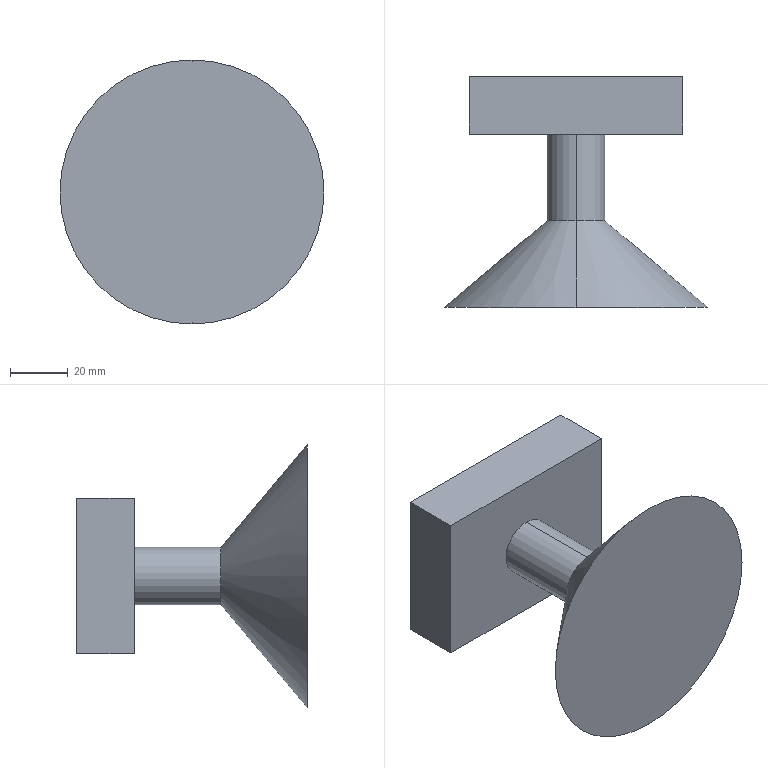Part | STEP file | Guide wheel mechanism revised.sldasm-Part-13 | 1 solid | 11 faces | box 91.505 x 80 x 91.505 mm | volume 172572 mm3 | plane 7 | cone 2 | cylinder 2 | commonest cylinder face diameters 20 x2
STEP:
#1=CARTESIAN_POINT('',(-444.995,-30.,-485.005));
#2=VERTEX_POINT('',#1);
#3=CARTESIAN_POINT('',(-444.995,-30.,-465.005));
#4=VERTEX_POINT('',#3);
#5=CARTESIAN_POINT('',(-444.995,-30.,-475.005));
#6=DIRECTION('',(0.,-1.,0.));
#7=DIRECTION('',(0.,0.,-1.));
#8=AXIS2_PLACEMENT_3D('',#5,#6,#7);
#9=CIRCLE('',#8,10.);
#10=EDGE_CURVE('',#2,#4,#9,.T.);
#11=ORIENTED_EDGE('',*,*,#10,.T.);
#12=CARTESIAN_POINT('',(-444.995,-60.,-429.252));
#13=VERTEX_POINT('',#12);
#14=CARTESIAN_POINT('',(-444.995,-30.,-465.005));
#15=DIRECTION('',(0.,-0.6428,0.766));
#16=VECTOR('',#15,1000.);
#17=LINE('',#14,#16);
#18=EDGE_CURVE('',#4,#13,#17,.T.);
#19=ORIENTED_EDGE('',*,*,#18,.T.);
#20=CARTESIAN_POINT('',(-444.995,-60.,-520.758));
#21=VERTEX_POINT('',#20);
#22=CARTESIAN_POINT('',(-444.995,-60.,-475.005));
#23=DIRECTION('',(0.,-1.,0.));
#24=DIRECTION('',(0.,0.,-1.));
#25=AXIS2_PLACEMENT_3D('',#22,#23,#24);
#26=CIRCLE('',#25,45.753);
#27=EDGE_CURVE('',#21,#13,#26,.T.);
#28=ORIENTED_EDGE('',*,*,#27,.F.);
#29=CARTESIAN_POINT('',(-444.995,-30.,-485.005));
#30=DIRECTION('',(0.,-0.6428,-0.766));
#31=VECTOR('',#30,1000.);
#32=LINE('',#29,#31);
#33=EDGE_CURVE('',#2,#21,#32,.T.);
#34=ORIENTED_EDGE('',*,*,#33,.F.);
#35=EDGE_LOOP('',(#11,#19,#28,#34));
#36=FACE_OUTER_BOUND('',#35,.T.);
#37=CARTESIAN_POINT('',(-444.995,-30.,-475.005));
#38=DIRECTION('',(0.,-1.,0.));
#39=DIRECTION('',(0.,0.,-1.));
#40=AXIS2_PLACEMENT_3D('',#37,#38,#39);
#41=CONICAL_SURFACE('',#40,10.,0.8727);
#42=ADVANCED_FACE('',(#36),#41,.T.);
#43=ORIENTED_EDGE('',*,*,#10,.F.);
#44=CARTESIAN_POINT('',(-444.995,0.,-485.005));
#45=VERTEX_POINT('',#44);
#46=CARTESIAN_POINT('',(-444.995,-30.,-485.005));
#47=DIRECTION('',(0.,1.,0.));
#48=VECTOR('',#47,1000.);
#49=LINE('',#46,#48);
#50=EDGE_CURVE('',#2,#45,#49,.T.);
#51=ORIENTED_EDGE('',*,*,#50,.T.);
#52=CARTESIAN_POINT('',(-444.995,0.,-465.005));
#53=VERTEX_POINT('',#52);
#54=CARTESIAN_POINT('',(-444.995,0.,-475.005));
#55=DIRECTION('',(0.,-1.,0.));
#56=DIRECTION('',(0.,0.,-1.));
#57=AXIS2_PLACEMENT_3D('',#54,#55,#56);
#58=CIRCLE('',#57,10.);
#59=EDGE_CURVE('',#45,#53,#58,.T.);
#60=ORIENTED_EDGE('',*,*,#59,.T.);
#61=CARTESIAN_POINT('',(-444.995,-30.,-465.005));
#62=DIRECTION('',(0.,1.,0.));
#63=VECTOR('',#62,1000.);
#64=LINE('',#61,#63);
#65=EDGE_CURVE('',#4,#53,#64,.T.);
#66=ORIENTED_EDGE('',*,*,#65,.F.);
#67=EDGE_LOOP('',(#43,#51,#60,#66));
#68=FACE_OUTER_BOUND('',#67,.T.);
#69=CARTESIAN_POINT('',(-444.995,-30.,-475.005));
#70=DIRECTION('',(0.,1.,0.));
#71=DIRECTION('',(0.,0.,1.));
#72=AXIS2_PLACEMENT_3D('',#69,#70,#71);
#73=CYLINDRICAL_SURFACE('',#72,10.);
#74=ADVANCED_FACE('',(#68),#73,.T.);
#75=CARTESIAN_POINT('',(-481.99,0.,-448.01));
#76=VERTEX_POINT('',#75);
#77=CARTESIAN_POINT('',(-481.99,0.,-501.99));
#78=VERTEX_POINT('',#77);
#79=CARTESIAN_POINT('',(-481.99,0.,-448.01));
#80=DIRECTION('',(0.,0.,-1.));
#81=VECTOR('',#80,1000.);
#82=LINE('',#79,#81);
#83=EDGE_CURVE('',#76,#78,#82,.T.);
#84=ORIENTED_EDGE('',*,*,#83,.T.);
#85=CARTESIAN_POINT('',(-408.01,0.,-501.99));
#86=VERTEX_POINT('',#85);
#87=CARTESIAN_POINT('',(-481.99,0.,-501.99));
#88=DIRECTION('',(1.,0.,0.));
#89=VECTOR('',#88,1000.);
#90=LINE('',#87,#89);
#91=EDGE_CURVE('',#78,#86,#90,.T.);
#92=ORIENTED_EDGE('',*,*,#91,.T.);
#93=CARTESIAN_POINT('',(-408.01,0.,-448.01));
#94=VERTEX_POINT('',#93);
#95=CARTESIAN_POINT('',(-408.01,0.,-448.01));
#96=DIRECTION('',(0.,0.,1.));
#97=VECTOR('',#96,1000.);
#98=LINE('',#95,#97);
#99=EDGE_CURVE('',#86,#94,#98,.T.);
#100=ORIENTED_EDGE('',*,*,#99,.T.);
#101=CARTESIAN_POINT('',(-481.99,0.,-448.01));
#102=DIRECTION('',(-1.,0.,0.));
#103=VECTOR('',#102,1000.);
#104=LINE('',#101,#103);
#105=EDGE_CURVE('',#94,#76,#104,.T.);
#106=ORIENTED_EDGE('',*,*,#105,.T.);
#107=EDGE_LOOP('',(#84,#92,#100,#106));
#108=FACE_OUTER_BOUND('',#107,.T.);
#109=CARTESIAN_POINT('',(-444.995,0.,-475.005));
#110=DIRECTION('',(0.,-1.,0.));
#111=DIRECTION('',(0.,0.,-1.));
#112=AXIS2_PLACEMENT_3D('',#109,#110,#111);
#113=CIRCLE('',#112,10.);
#114=EDGE_CURVE('',#53,#45,#113,.T.);
#115=ORIENTED_EDGE('',*,*,#114,.F.);
#116=ORIENTED_EDGE('',*,*,#59,.F.);
#117=EDGE_LOOP('',(#115,#116));
#118=FACE_BOUND('',#117,.T.);
#119=CARTESIAN_POINT('',(0.,0.,0.));
#120=DIRECTION('',(0.,-1.,0.));
#121=DIRECTION('',(0.,0.,-1.));
#122=AXIS2_PLACEMENT_3D('',#119,#120,#121);
#123=PLANE('',#122);
#124=ADVANCED_FACE('',(#108,#118),#123,.T.);
#125=ORIENTED_EDGE('',*,*,#83,.F.);
#126=CARTESIAN_POINT('',(-481.99,20.,-448.01));
#127=VERTEX_POINT('',#126);
#128=CARTESIAN_POINT('',(-481.99,20.,-448.01));
#129=DIRECTION('',(0.,-1.,0.));
#130=VECTOR('',#129,1000.);
#131=LINE('',#128,#130);
#132=EDGE_CURVE('',#127,#76,#131,.T.);
#133=ORIENTED_EDGE('',*,*,#132,.F.);
#134=CARTESIAN_POINT('',(-481.99,20.,-501.99));
#135=VERTEX_POINT('',#134);
#136=CARTESIAN_POINT('',(-481.99,20.,-448.01));
#137=DIRECTION('',(0.,0.,-1.));
#138=VECTOR('',#137,1000.);
#139=LINE('',#136,#138);
#140=EDGE_CURVE('',#127,#135,#139,.T.);
#141=ORIENTED_EDGE('',*,*,#140,.T.);
#142=CARTESIAN_POINT('',(-481.99,20.,-501.99));
#143=DIRECTION('',(0.,-1.,0.));
#144=VECTOR('',#143,1000.);
#145=LINE('',#142,#144);
#146=EDGE_CURVE('',#135,#78,#145,.T.);
#147=ORIENTED_EDGE('',*,*,#146,.T.);
#148=EDGE_LOOP('',(#125,#133,#141,#147));
#149=FACE_OUTER_BOUND('',#148,.T.);
#150=CARTESIAN_POINT('',(-481.99,20.,-448.01));
#151=DIRECTION('',(-1.,0.,0.));
#152=DIRECTION('',(0.,0.,1.));
#153=AXIS2_PLACEMENT_3D('',#150,#151,#152);
#154=PLANE('',#153);
#155=ADVANCED_FACE('',(#149),#154,.T.);
#156=ORIENTED_EDGE('',*,*,#105,.F.);
#157=CARTESIAN_POINT('',(-408.01,20.,-448.01));
#158=VERTEX_POINT('',#157);
#159=CARTESIAN_POINT('',(-408.01,20.,-448.01));
#160=DIRECTION('',(0.,-1.,0.));
#161=VECTOR('',#160,1000.);
#162=LINE('',#159,#161);
#163=EDGE_CURVE('',#158,#94,#162,.T.);
#164=ORIENTED_EDGE('',*,*,#163,.F.);
#165=CARTESIAN_POINT('',(-481.99,20.,-448.01));
#166=DIRECTION('',(-1.,0.,0.));
#167=VECTOR('',#166,1000.);
#168=LINE('',#165,#167);
#169=EDGE_CURVE('',#158,#127,#168,.T.);
#170=ORIENTED_EDGE('',*,*,#169,.T.);
#171=ORIENTED_EDGE('',*,*,#132,.T.);
#172=EDGE_LOOP('',(#156,#164,#170,#171));
#173=FACE_OUTER_BOUND('',#172,.T.);
#174=CARTESIAN_POINT('',(-481.99,20.,-448.01));
#175=DIRECTION('',(0.,0.,1.));
#176=DIRECTION('',(1.,0.,0.));
#177=AXIS2_PLACEMENT_3D('',#174,#175,#176);
#178=PLANE('',#177);
#179=ADVANCED_FACE('',(#173),#178,.T.);
#180=ORIENTED_EDGE('',*,*,#99,.F.);
#181=CARTESIAN_POINT('',(-408.01,20.,-501.99));
#182=VERTEX_POINT('',#181);
#183=CARTESIAN_POINT('',(-408.01,20.,-501.99));
#184=DIRECTION('',(0.,-1.,0.));
#185=VECTOR('',#184,1000.);
#186=LINE('',#183,#185);
#187=EDGE_CURVE('',#182,#86,#186,.T.);
#188=ORIENTED_EDGE('',*,*,#187,.F.);
#189=CARTESIAN_POINT('',(-408.01,20.,-448.01));
#190=DIRECTION('',(0.,0.,1.));
#191=VECTOR('',#190,1000.);
#192=LINE('',#189,#191);
#193=EDGE_CURVE('',#182,#158,#192,.T.);
#194=ORIENTED_EDGE('',*,*,#193,.T.);
#195=ORIENTED_EDGE('',*,*,#163,.T.);
#196=EDGE_LOOP('',(#180,#188,#194,#195));
#197=FACE_OUTER_BOUND('',#196,.T.);
#198=CARTESIAN_POINT('',(-408.01,20.,-448.01));
#199=DIRECTION('',(1.,0.,0.));
#200=DIRECTION('',(0.,0.,-1.));
#201=AXIS2_PLACEMENT_3D('',#198,#199,#200);
#202=PLANE('',#201);
#203=ADVANCED_FACE('',(#197),#202,.T.);
#204=ORIENTED_EDGE('',*,*,#91,.F.);
#205=ORIENTED_EDGE('',*,*,#146,.F.);
#206=CARTESIAN_POINT('',(-481.99,20.,-501.99));
#207=DIRECTION('',(1.,0.,0.));
#208=VECTOR('',#207,1000.);
#209=LINE('',#206,#208);
#210=EDGE_CURVE('',#135,#182,#209,.T.);
#211=ORIENTED_EDGE('',*,*,#210,.T.);
#212=ORIENTED_EDGE('',*,*,#187,.T.);
#213=EDGE_LOOP('',(#204,#205,#211,#212));
#214=FACE_OUTER_BOUND('',#213,.T.);
#215=CARTESIAN_POINT('',(-481.99,20.,-501.99));
#216=DIRECTION('',(0.,0.,-1.));
#217=DIRECTION('',(-1.,0.,0.));
#218=AXIS2_PLACEMENT_3D('',#215,#216,#217);
#219=PLANE('',#218);
#220=ADVANCED_FACE('',(#214),#219,.T.);
#221=ORIENTED_EDGE('',*,*,#140,.F.);
#222=ORIENTED_EDGE('',*,*,#169,.F.);
#223=ORIENTED_EDGE('',*,*,#193,.F.);
#224=ORIENTED_EDGE('',*,*,#210,.F.);
#225=EDGE_LOOP('',(#221,#222,#223,#224));
#226=FACE_OUTER_BOUND('',#225,.T.);
#227=CARTESIAN_POINT('',(0.,20.,0.));
#228=DIRECTION('',(0.,-1.,0.));
#229=DIRECTION('',(0.,0.,-1.));
#230=AXIS2_PLACEMENT_3D('',#227,#228,#229);
#231=PLANE('',#230);
#232=ADVANCED_FACE('',(#226),#231,.F.);
#233=ORIENTED_EDGE('',*,*,#50,.F.);
#234=CARTESIAN_POINT('',(-444.995,-30.,-475.005));
#235=DIRECTION('',(0.,-1.,0.));
#236=DIRECTION('',(0.,0.,-1.));
#237=AXIS2_PLACEMENT_3D('',#234,#235,#236);
#238=CIRCLE('',#237,10.);
#239=EDGE_CURVE('',#4,#2,#238,.T.);
#240=ORIENTED_EDGE('',*,*,#239,.F.);
#241=ORIENTED_EDGE('',*,*,#65,.T.);
#242=ORIENTED_EDGE('',*,*,#114,.T.);
#243=EDGE_LOOP('',(#233,#240,#241,#242));
#244=FACE_OUTER_BOUND('',#243,.T.);
#245=CARTESIAN_POINT('',(-444.995,-30.,-475.005));
#246=DIRECTION('',(0.,1.,0.));
#247=DIRECTION('',(0.,0.,1.));
#248=AXIS2_PLACEMENT_3D('',#245,#246,#247);
#249=CYLINDRICAL_SURFACE('',#248,10.);
#250=ADVANCED_FACE('',(#244),#249,.T.);
#251=ORIENTED_EDGE('',*,*,#18,.F.);
#252=ORIENTED_EDGE('',*,*,#239,.T.);
#253=ORIENTED_EDGE('',*,*,#33,.T.);
#254=CARTESIAN_POINT('',(-444.995,-60.,-475.005));
#255=DIRECTION('',(0.,-1.,0.));
#256=DIRECTION('',(0.,0.,-1.));
#257=AXIS2_PLACEMENT_3D('',#254,#255,#256);
#258=CIRCLE('',#257,45.753);
#259=EDGE_CURVE('',#13,#21,#258,.T.);
#260=ORIENTED_EDGE('',*,*,#259,.F.);
#261=EDGE_LOOP('',(#251,#252,#253,#260));
#262=FACE_OUTER_BOUND('',#261,.T.);
#263=CARTESIAN_POINT('',(-444.995,-30.,-475.005));
#264=DIRECTION('',(0.,-1.,0.));
#265=DIRECTION('',(0.,0.,-1.));
#266=AXIS2_PLACEMENT_3D('',#263,#264,#265);
#267=CONICAL_SURFACE('',#266,10.,0.8727);
#268=ADVANCED_FACE('',(#262),#267,.T.);
#269=ORIENTED_EDGE('',*,*,#27,.T.);
#270=ORIENTED_EDGE('',*,*,#259,.T.);
#271=EDGE_LOOP('',(#269,#270));
#272=FACE_OUTER_BOUND('',#271,.T.);
#273=CARTESIAN_POINT('',(-444.995,-60.,-475.005));
#274=DIRECTION('',(0.,-1.,0.));
#275=DIRECTION('',(0.,0.,-1.));
#276=AXIS2_PLACEMENT_3D('',#273,#274,#275);
#277=PLANE('',#276);
#278=ADVANCED_FACE('',(#272),#277,.T.);
#279=CLOSED_SHELL('',(#42,#74,#124,#155,#179,#203,#220,#232,#250,#268,#278));
#280=MANIFOLD_SOLID_BREP('',#279);
#281=CARTESIAN_POINT('',(0.,0.,0.));
#282=DIRECTION('',(0.,0.,1.));
#283=DIRECTION('',(1.,0.,0.));
#284=AXIS2_PLACEMENT_3D('',#281,#282,#283);
#285=(LENGTH_UNIT()NAMED_UNIT(*)SI_UNIT(.MILLI.,.METRE.));
#286=UNCERTAINTY_MEASURE_WITH_UNIT(LENGTH_MEASURE(0.00001),#285,'','');
#287=(NAMED_UNIT(*)PLANE_ANGLE_UNIT()SI_UNIT($,.RADIAN.));
#288=(NAMED_UNIT(*)SI_UNIT($,.STERADIAN.)SOLID_ANGLE_UNIT());
#289=(GEOMETRIC_REPRESENTATION_CONTEXT(3)GLOBAL_UNCERTAINTY_ASSIGNED_CONTEXT((#286))GLOBAL_UNIT_ASSIGNED_CONTEXT((#285,#287,#288))REPRESENTATION_CONTEXT('',''));
#290=ADVANCED_BREP_SHAPE_REPRESENTATION('',(#280,#284),#289);